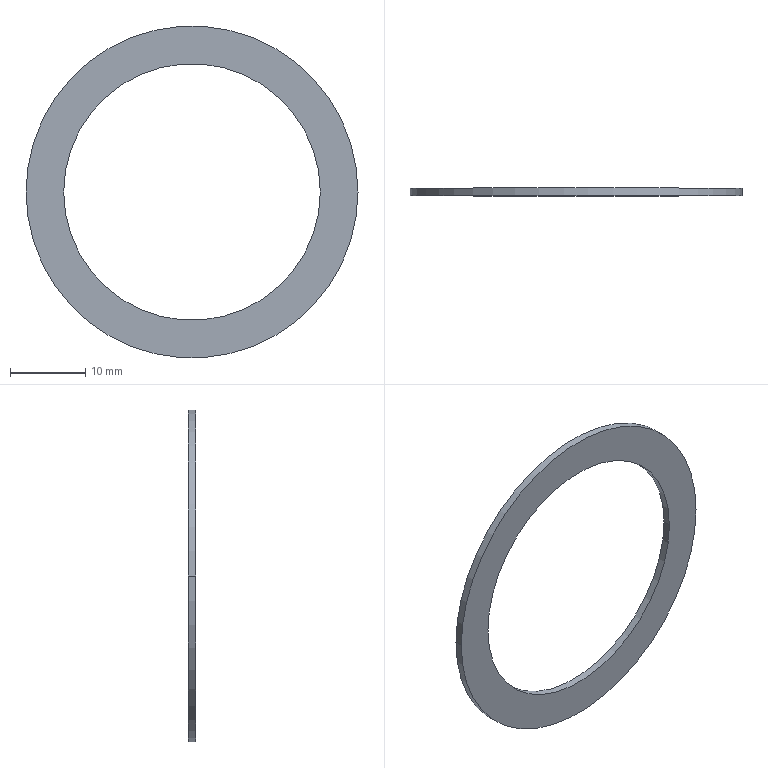Part | STEP file | MSBR-32 | 1 solid | 6 faces | box 44 x 1 x 44 mm | volume 612.611 mm3 | cylinder 4 | plane 2 | commonest cylinder face diameters 34 x2 44 x2
STEP:
#1=CARTESIAN_POINT('',(0.,0.,0.));
#2=DIRECTION('',(0.,0.,1.));
#3=DIRECTION('',(1.,0.,0.));
#4=AXIS2_PLACEMENT_3D('',#1,#2,#3);
#5=CARTESIAN_POINT('',(22.,-93.83,0.1));
#6=VERTEX_POINT('',#5);
#7=CARTESIAN_POINT('',(-22.,-93.83,0.1));
#8=VERTEX_POINT('',#7);
#9=CARTESIAN_POINT('',(0.,-93.83,0.1));
#10=DIRECTION('',(0.,-1.,0.));
#11=DIRECTION('',(1.,0.,0.));
#12=AXIS2_PLACEMENT_3D('',#9,#10,#11);
#13=CIRCLE('',#12,22.);
#14=EDGE_CURVE('',#6,#8,#13,.T.);
#15=ORIENTED_EDGE('',*,*,#14,.T.);
#16=CARTESIAN_POINT('',(0.,-93.83,0.1));
#17=DIRECTION('',(0.,-1.,0.));
#18=DIRECTION('',(-1.,0.,0.));
#19=AXIS2_PLACEMENT_3D('',#16,#17,#18);
#20=CIRCLE('',#19,22.);
#21=EDGE_CURVE('',#8,#6,#20,.T.);
#22=ORIENTED_EDGE('',*,*,#21,.T.);
#23=EDGE_LOOP('',(#15,#22));
#24=FACE_OUTER_BOUND('',#23,.F.);
#25=CARTESIAN_POINT('',(17.,-93.83,0.1));
#26=VERTEX_POINT('',#25);
#27=CARTESIAN_POINT('',(-17.,-93.83,0.1));
#28=VERTEX_POINT('',#27);
#29=CARTESIAN_POINT('',(0.,-93.83,0.1));
#30=DIRECTION('',(0.,1.,0.));
#31=DIRECTION('',(1.,0.,0.));
#32=AXIS2_PLACEMENT_3D('',#29,#30,#31);
#33=CIRCLE('',#32,17.);
#34=EDGE_CURVE('',#26,#28,#33,.T.);
#35=ORIENTED_EDGE('',*,*,#34,.T.);
#36=CARTESIAN_POINT('',(0.,-93.83,0.1));
#37=DIRECTION('',(0.,1.,0.));
#38=DIRECTION('',(-1.,0.,0.));
#39=AXIS2_PLACEMENT_3D('',#36,#37,#38);
#40=CIRCLE('',#39,17.);
#41=EDGE_CURVE('',#28,#26,#40,.T.);
#42=ORIENTED_EDGE('',*,*,#41,.T.);
#43=EDGE_LOOP('',(#35,#42));
#44=FACE_BOUND('',#43,.F.);
#45=CARTESIAN_POINT('',(0.,-93.83,0.1));
#46=DIRECTION('',(0.,1.,0.));
#47=DIRECTION('',(1.,0.,0.));
#48=AXIS2_PLACEMENT_3D('',#45,#46,#47);
#49=PLANE('',#48);
#50=ADVANCED_FACE('',(#24,#44),#49,.T.);
#51=ORIENTED_EDGE('',*,*,#14,.F.);
#52=CARTESIAN_POINT('',(22.,-94.83,0.1));
#53=VERTEX_POINT('',#52);
#54=CARTESIAN_POINT('',(22.,-94.83,0.1));
#55=DIRECTION('',(0.,1.,0.));
#56=VECTOR('',#55,1.);
#57=LINE('',#54,#56);
#58=EDGE_CURVE('',#53,#6,#57,.T.);
#59=ORIENTED_EDGE('',*,*,#58,.F.);
#60=CARTESIAN_POINT('',(-22.,-94.83,0.1));
#61=VERTEX_POINT('',#60);
#62=CARTESIAN_POINT('',(0.,-94.83,0.1));
#63=DIRECTION('',(0.,1.,0.));
#64=DIRECTION('',(-1.,0.,0.));
#65=AXIS2_PLACEMENT_3D('',#62,#63,#64);
#66=CIRCLE('',#65,22.);
#67=EDGE_CURVE('',#61,#53,#66,.T.);
#68=ORIENTED_EDGE('',*,*,#67,.F.);
#69=CARTESIAN_POINT('',(-22.,-93.83,0.1));
#70=DIRECTION('',(0.,-1.,0.));
#71=VECTOR('',#70,1.);
#72=LINE('',#69,#71);
#73=EDGE_CURVE('',#8,#61,#72,.T.);
#74=ORIENTED_EDGE('',*,*,#73,.F.);
#75=EDGE_LOOP('',(#51,#59,#68,#74));
#76=FACE_OUTER_BOUND('',#75,.F.);
#77=CARTESIAN_POINT('',(0.,-93.755,0.1));
#78=DIRECTION('',(0.,-1.,0.));
#79=DIRECTION('',(1.,0.,0.));
#80=AXIS2_PLACEMENT_3D('',#77,#78,#79);
#81=CYLINDRICAL_SURFACE('',#80,22.);
#82=ADVANCED_FACE('',(#76),#81,.T.);
#83=ORIENTED_EDGE('',*,*,#21,.F.);
#84=ORIENTED_EDGE('',*,*,#73,.T.);
#85=CARTESIAN_POINT('',(0.,-94.83,0.1));
#86=DIRECTION('',(0.,1.,0.));
#87=DIRECTION('',(1.,0.,0.));
#88=AXIS2_PLACEMENT_3D('',#85,#86,#87);
#89=CIRCLE('',#88,22.);
#90=EDGE_CURVE('',#53,#61,#89,.T.);
#91=ORIENTED_EDGE('',*,*,#90,.F.);
#92=ORIENTED_EDGE('',*,*,#58,.T.);
#93=EDGE_LOOP('',(#83,#84,#91,#92));
#94=FACE_OUTER_BOUND('',#93,.F.);
#95=CARTESIAN_POINT('',(0.,-93.755,0.1));
#96=DIRECTION('',(0.,-1.,0.));
#97=DIRECTION('',(1.,0.,0.));
#98=AXIS2_PLACEMENT_3D('',#95,#96,#97);
#99=CYLINDRICAL_SURFACE('',#98,22.);
#100=ADVANCED_FACE('',(#94),#99,.T.);
#101=ORIENTED_EDGE('',*,*,#67,.T.);
#102=ORIENTED_EDGE('',*,*,#90,.T.);
#103=EDGE_LOOP('',(#101,#102));
#104=FACE_OUTER_BOUND('',#103,.F.);
#105=CARTESIAN_POINT('',(-17.,-94.83,0.1));
#106=VERTEX_POINT('',#105);
#107=CARTESIAN_POINT('',(17.,-94.83,0.1));
#108=VERTEX_POINT('',#107);
#109=CARTESIAN_POINT('',(0.,-94.83,0.1));
#110=DIRECTION('',(0.,-1.,0.));
#111=DIRECTION('',(-1.,0.,0.));
#112=AXIS2_PLACEMENT_3D('',#109,#110,#111);
#113=CIRCLE('',#112,17.);
#114=EDGE_CURVE('',#106,#108,#113,.T.);
#115=ORIENTED_EDGE('',*,*,#114,.T.);
#116=CARTESIAN_POINT('',(0.,-94.83,0.1));
#117=DIRECTION('',(0.,-1.,0.));
#118=DIRECTION('',(1.,0.,0.));
#119=AXIS2_PLACEMENT_3D('',#116,#117,#118);
#120=CIRCLE('',#119,17.);
#121=EDGE_CURVE('',#108,#106,#120,.T.);
#122=ORIENTED_EDGE('',*,*,#121,.T.);
#123=EDGE_LOOP('',(#115,#122));
#124=FACE_BOUND('',#123,.F.);
#125=CARTESIAN_POINT('',(0.,-94.83,0.1));
#126=DIRECTION('',(0.,1.,0.));
#127=DIRECTION('',(1.,0.,0.));
#128=AXIS2_PLACEMENT_3D('',#125,#126,#127);
#129=PLANE('',#128);
#130=ADVANCED_FACE('',(#104,#124),#129,.F.);
#131=ORIENTED_EDGE('',*,*,#34,.F.);
#132=CARTESIAN_POINT('',(17.,-94.83,0.1));
#133=DIRECTION('',(0.,1.,0.));
#134=VECTOR('',#133,1.);
#135=LINE('',#132,#134);
#136=EDGE_CURVE('',#108,#26,#135,.T.);
#137=ORIENTED_EDGE('',*,*,#136,.F.);
#138=ORIENTED_EDGE('',*,*,#114,.F.);
#139=CARTESIAN_POINT('',(-17.,-93.83,0.1));
#140=DIRECTION('',(0.,-1.,0.));
#141=VECTOR('',#140,1.);
#142=LINE('',#139,#141);
#143=EDGE_CURVE('',#28,#106,#142,.T.);
#144=ORIENTED_EDGE('',*,*,#143,.F.);
#145=EDGE_LOOP('',(#131,#137,#138,#144));
#146=FACE_OUTER_BOUND('',#145,.F.);
#147=CARTESIAN_POINT('',(0.,-93.755,0.1));
#148=DIRECTION('',(0.,-1.,0.));
#149=DIRECTION('',(1.,0.,0.));
#150=AXIS2_PLACEMENT_3D('',#147,#148,#149);
#151=CYLINDRICAL_SURFACE('',#150,17.);
#152=ADVANCED_FACE('',(#146),#151,.F.);
#153=ORIENTED_EDGE('',*,*,#41,.F.);
#154=ORIENTED_EDGE('',*,*,#143,.T.);
#155=ORIENTED_EDGE('',*,*,#121,.F.);
#156=ORIENTED_EDGE('',*,*,#136,.T.);
#157=EDGE_LOOP('',(#153,#154,#155,#156));
#158=FACE_OUTER_BOUND('',#157,.F.);
#159=CARTESIAN_POINT('',(0.,-93.755,0.1));
#160=DIRECTION('',(0.,-1.,0.));
#161=DIRECTION('',(1.,0.,0.));
#162=AXIS2_PLACEMENT_3D('',#159,#160,#161);
#163=CYLINDRICAL_SURFACE('',#162,17.);
#164=ADVANCED_FACE('',(#158),#163,.F.);
#165=CLOSED_SHELL('',(#50,#82,#100,#130,#152,#164));
#166=MANIFOLD_SOLID_BREP('',#165);
#167=(LENGTH_UNIT()NAMED_UNIT(*)SI_UNIT(.MILLI.,.METRE.));
#168=UNCERTAINTY_MEASURE_WITH_UNIT(LENGTH_MEASURE(0.006225),#167,'','');
#169=(NAMED_UNIT(*)PLANE_ANGLE_UNIT()SI_UNIT($,.RADIAN.));
#170=PLANE_ANGLE_MEASURE_WITH_UNIT(PLANE_ANGLE_MEASURE(0.01745),#169);
#171=(CONVERSION_BASED_UNIT('DEGREE',#170)NAMED_UNIT(*)PLANE_ANGLE_UNIT());
#172=(NAMED_UNIT(*)SI_UNIT($,.STERADIAN.)SOLID_ANGLE_UNIT());
#173=(GEOMETRIC_REPRESENTATION_CONTEXT(3)GLOBAL_UNCERTAINTY_ASSIGNED_CONTEXT((#168))GLOBAL_UNIT_ASSIGNED_CONTEXT((#167,#171,#172))REPRESENTATION_CONTEXT('',''));
#174=ADVANCED_BREP_SHAPE_REPRESENTATION('',(#4,#166),#173);